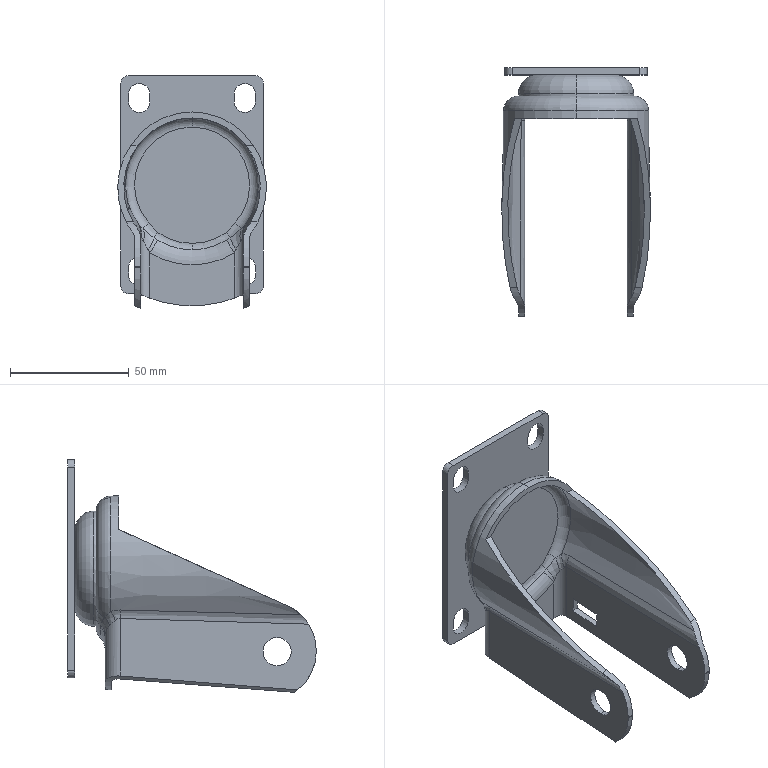Part | SolidWorks | features ICE 8, Fillet 5, Extrusion 1, RevCut 1, Revolution 1, Shell 1 | 1 solid | 111 faces | box 62.612 x 104.648 x 97.984 mm | volume 58421 mm3 | plane 33 | cylinder 32 | spline 24 | torus 16 | cone 6 | commonest cylinder face diameters 9.017 x12 6.35 x4 11.852 x4 41.275 x4 7.62 x2 12.7 x2